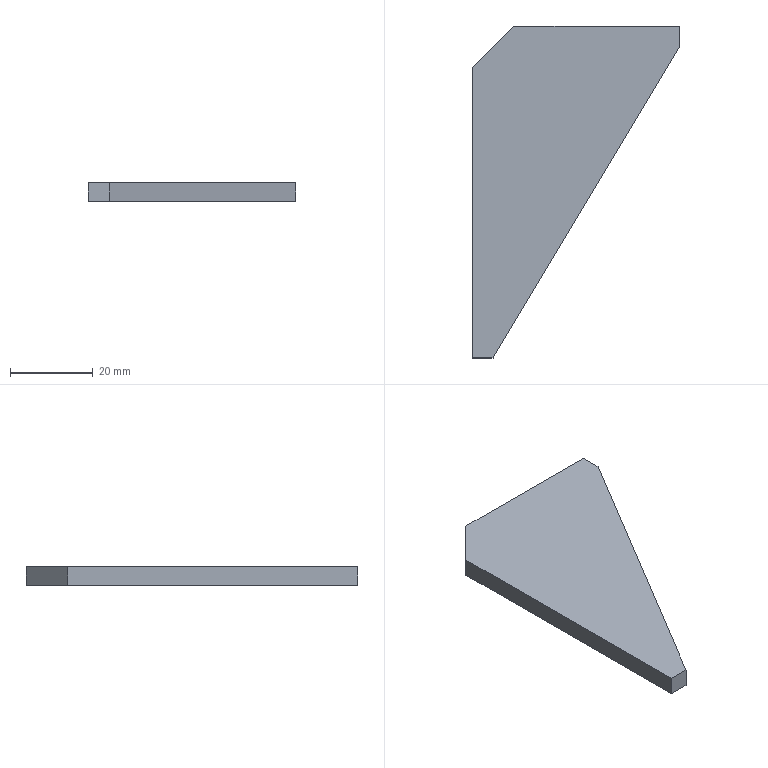Part | SolidWorks | features FlatPattern 1, SMBaseFlange 1, SheetMetal 1 | 1 solid | 8 faces | box 50 x 80 x 4.5 mm | volume 10181 mm3 | plane 8
STEP:
#1=CARTESIAN_POINT('',(0.,-5.,0.));
#2=VERTEX_POINT('',#1);
#3=CARTESIAN_POINT('',(0.,0.,0.));
#4=VERTEX_POINT('',#3);
#5=CARTESIAN_POINT('',(0.,-5.,0.));
#6=DIRECTION('',(0.,1.,0.));
#7=VECTOR('',#6,1000.);
#8=LINE('',#5,#7);
#9=EDGE_CURVE('',#2,#4,#8,.T.);
#10=ORIENTED_EDGE('',*,*,#9,.F.);
#11=CARTESIAN_POINT('',(0.,-5.,-4.5));
#12=VERTEX_POINT('',#11);
#13=CARTESIAN_POINT('',(0.,-5.,-4.5));
#14=DIRECTION('',(0.,0.,1.));
#15=VECTOR('',#14,1000.);
#16=LINE('',#13,#15);
#17=EDGE_CURVE('',#12,#2,#16,.T.);
#18=ORIENTED_EDGE('',*,*,#17,.F.);
#19=CARTESIAN_POINT('',(0.,0.,-4.5));
#20=VERTEX_POINT('',#19);
#21=CARTESIAN_POINT('',(0.,-5.,-4.5));
#22=DIRECTION('',(0.,1.,0.));
#23=VECTOR('',#22,1000.);
#24=LINE('',#21,#23);
#25=EDGE_CURVE('',#12,#20,#24,.T.);
#26=ORIENTED_EDGE('',*,*,#25,.T.);
#27=CARTESIAN_POINT('',(0.,0.,-4.5));
#28=DIRECTION('',(0.,0.,1.));
#29=VECTOR('',#28,1000.);
#30=LINE('',#27,#29);
#31=EDGE_CURVE('',#20,#4,#30,.T.);
#32=ORIENTED_EDGE('',*,*,#31,.T.);
#33=EDGE_LOOP('',(#10,#18,#26,#32));
#34=FACE_OUTER_BOUND('',#33,.T.);
#35=CARTESIAN_POINT('',(0.,-5.,-4.5));
#36=DIRECTION('',(1.,0.,0.));
#37=DIRECTION('',(0.,0.,-1.));
#38=AXIS2_PLACEMENT_3D('',#35,#36,#37);
#39=PLANE('',#38);
#40=ADVANCED_FACE('',(#34),#39,.T.);
#41=CARTESIAN_POINT('',(-45.,-80.,0.));
#42=VERTEX_POINT('',#41);
#43=CARTESIAN_POINT('',(-45.,-80.,0.));
#44=DIRECTION('',(0.5145,0.8575,0.));
#45=VECTOR('',#44,1000.);
#46=LINE('',#43,#45);
#47=EDGE_CURVE('',#42,#2,#46,.T.);
#48=ORIENTED_EDGE('',*,*,#47,.F.);
#49=CARTESIAN_POINT('',(-45.,-80.,-4.5));
#50=VERTEX_POINT('',#49);
#51=CARTESIAN_POINT('',(-45.,-80.,-4.5));
#52=DIRECTION('',(0.,0.,1.));
#53=VECTOR('',#52,1000.);
#54=LINE('',#51,#53);
#55=EDGE_CURVE('',#50,#42,#54,.T.);
#56=ORIENTED_EDGE('',*,*,#55,.F.);
#57=CARTESIAN_POINT('',(-45.,-80.,-4.5));
#58=DIRECTION('',(0.5145,0.8575,0.));
#59=VECTOR('',#58,1000.);
#60=LINE('',#57,#59);
#61=EDGE_CURVE('',#50,#12,#60,.T.);
#62=ORIENTED_EDGE('',*,*,#61,.T.);
#63=ORIENTED_EDGE('',*,*,#17,.T.);
#64=EDGE_LOOP('',(#48,#56,#62,#63));
#65=FACE_OUTER_BOUND('',#64,.T.);
#66=CARTESIAN_POINT('',(-45.,-80.,-4.5));
#67=DIRECTION('',(0.8575,-0.5145,0.));
#68=DIRECTION('',(0.5145,0.8575,0.));
#69=AXIS2_PLACEMENT_3D('',#66,#67,#68);
#70=PLANE('',#69);
#71=ADVANCED_FACE('',(#65),#70,.T.);
#72=CARTESIAN_POINT('',(-50.,-80.,0.));
#73=VERTEX_POINT('',#72);
#74=CARTESIAN_POINT('',(-50.,-80.,0.));
#75=DIRECTION('',(1.,0.,0.));
#76=VECTOR('',#75,1000.);
#77=LINE('',#74,#76);
#78=EDGE_CURVE('',#73,#42,#77,.T.);
#79=ORIENTED_EDGE('',*,*,#78,.F.);
#80=CARTESIAN_POINT('',(-50.,-80.,-4.5));
#81=VERTEX_POINT('',#80);
#82=CARTESIAN_POINT('',(-50.,-80.,-4.5));
#83=DIRECTION('',(0.,0.,1.));
#84=VECTOR('',#83,1000.);
#85=LINE('',#82,#84);
#86=EDGE_CURVE('',#81,#73,#85,.T.);
#87=ORIENTED_EDGE('',*,*,#86,.F.);
#88=CARTESIAN_POINT('',(-50.,-80.,-4.5));
#89=DIRECTION('',(1.,0.,0.));
#90=VECTOR('',#89,1000.);
#91=LINE('',#88,#90);
#92=EDGE_CURVE('',#81,#50,#91,.T.);
#93=ORIENTED_EDGE('',*,*,#92,.T.);
#94=ORIENTED_EDGE('',*,*,#55,.T.);
#95=EDGE_LOOP('',(#79,#87,#93,#94));
#96=FACE_OUTER_BOUND('',#95,.T.);
#97=CARTESIAN_POINT('',(-50.,-80.,-4.5));
#98=DIRECTION('',(0.,-1.,0.));
#99=DIRECTION('',(0.,0.,-1.));
#100=AXIS2_PLACEMENT_3D('',#97,#98,#99);
#101=PLANE('',#100);
#102=ADVANCED_FACE('',(#96),#101,.T.);
#103=CARTESIAN_POINT('',(-50.,-10.,0.));
#104=VERTEX_POINT('',#103);
#105=CARTESIAN_POINT('',(-50.,-10.,0.));
#106=DIRECTION('',(0.,-1.,0.));
#107=VECTOR('',#106,1000.);
#108=LINE('',#105,#107);
#109=EDGE_CURVE('',#104,#73,#108,.T.);
#110=ORIENTED_EDGE('',*,*,#109,.F.);
#111=CARTESIAN_POINT('',(-50.,-10.,-4.5));
#112=VERTEX_POINT('',#111);
#113=CARTESIAN_POINT('',(-50.,-10.,-4.5));
#114=DIRECTION('',(0.,0.,1.));
#115=VECTOR('',#114,1000.);
#116=LINE('',#113,#115);
#117=EDGE_CURVE('',#112,#104,#116,.T.);
#118=ORIENTED_EDGE('',*,*,#117,.F.);
#119=CARTESIAN_POINT('',(-50.,-10.,-4.5));
#120=DIRECTION('',(0.,-1.,0.));
#121=VECTOR('',#120,1000.);
#122=LINE('',#119,#121);
#123=EDGE_CURVE('',#112,#81,#122,.T.);
#124=ORIENTED_EDGE('',*,*,#123,.T.);
#125=ORIENTED_EDGE('',*,*,#86,.T.);
#126=EDGE_LOOP('',(#110,#118,#124,#125));
#127=FACE_OUTER_BOUND('',#126,.T.);
#128=CARTESIAN_POINT('',(-50.,-10.,-4.5));
#129=DIRECTION('',(-1.,0.,0.));
#130=DIRECTION('',(0.,-1.,0.));
#131=AXIS2_PLACEMENT_3D('',#128,#129,#130);
#132=PLANE('',#131);
#133=ADVANCED_FACE('',(#127),#132,.T.);
#134=CARTESIAN_POINT('',(-40.,0.,0.));
#135=VERTEX_POINT('',#134);
#136=CARTESIAN_POINT('',(-40.,0.,0.));
#137=DIRECTION('',(-0.7071,-0.7071,0.));
#138=VECTOR('',#137,1000.);
#139=LINE('',#136,#138);
#140=EDGE_CURVE('',#135,#104,#139,.T.);
#141=ORIENTED_EDGE('',*,*,#140,.F.);
#142=CARTESIAN_POINT('',(-40.,0.,-4.5));
#143=VERTEX_POINT('',#142);
#144=CARTESIAN_POINT('',(-40.,0.,-4.5));
#145=DIRECTION('',(0.,0.,1.));
#146=VECTOR('',#145,1000.);
#147=LINE('',#144,#146);
#148=EDGE_CURVE('',#143,#135,#147,.T.);
#149=ORIENTED_EDGE('',*,*,#148,.F.);
#150=CARTESIAN_POINT('',(-40.,0.,-4.5));
#151=DIRECTION('',(-0.7071,-0.7071,0.));
#152=VECTOR('',#151,1000.);
#153=LINE('',#150,#152);
#154=EDGE_CURVE('',#143,#112,#153,.T.);
#155=ORIENTED_EDGE('',*,*,#154,.T.);
#156=ORIENTED_EDGE('',*,*,#117,.T.);
#157=EDGE_LOOP('',(#141,#149,#155,#156));
#158=FACE_OUTER_BOUND('',#157,.T.);
#159=CARTESIAN_POINT('',(-40.,0.,-4.5));
#160=DIRECTION('',(-0.7071,0.7071,0.));
#161=DIRECTION('',(-0.7071,-0.7071,0.));
#162=AXIS2_PLACEMENT_3D('',#159,#160,#161);
#163=PLANE('',#162);
#164=ADVANCED_FACE('',(#158),#163,.T.);
#165=CARTESIAN_POINT('',(0.,0.,0.));
#166=DIRECTION('',(-1.,0.,0.));
#167=VECTOR('',#166,1000.);
#168=LINE('',#165,#167);
#169=EDGE_CURVE('',#4,#135,#168,.T.);
#170=ORIENTED_EDGE('',*,*,#169,.F.);
#171=ORIENTED_EDGE('',*,*,#31,.F.);
#172=CARTESIAN_POINT('',(0.,0.,-4.5));
#173=DIRECTION('',(-1.,0.,0.));
#174=VECTOR('',#173,1000.);
#175=LINE('',#172,#174);
#176=EDGE_CURVE('',#20,#143,#175,.T.);
#177=ORIENTED_EDGE('',*,*,#176,.T.);
#178=ORIENTED_EDGE('',*,*,#148,.T.);
#179=EDGE_LOOP('',(#170,#171,#177,#178));
#180=FACE_OUTER_BOUND('',#179,.T.);
#181=CARTESIAN_POINT('',(0.,0.,-4.5));
#182=DIRECTION('',(0.,1.,0.));
#183=DIRECTION('',(0.,0.,1.));
#184=AXIS2_PLACEMENT_3D('',#181,#182,#183);
#185=PLANE('',#184);
#186=ADVANCED_FACE('',(#180),#185,.T.);
#187=ORIENTED_EDGE('',*,*,#25,.F.);
#188=ORIENTED_EDGE('',*,*,#61,.F.);
#189=ORIENTED_EDGE('',*,*,#92,.F.);
#190=ORIENTED_EDGE('',*,*,#123,.F.);
#191=ORIENTED_EDGE('',*,*,#154,.F.);
#192=ORIENTED_EDGE('',*,*,#176,.F.);
#193=EDGE_LOOP('',(#187,#188,#189,#190,#191,#192));
#194=FACE_OUTER_BOUND('',#193,.T.);
#195=CARTESIAN_POINT('',(0.,0.,-4.5));
#196=DIRECTION('',(0.,0.,1.));
#197=DIRECTION('',(1.,0.,0.));
#198=AXIS2_PLACEMENT_3D('',#195,#196,#197);
#199=PLANE('',#198);
#200=ADVANCED_FACE('',(#194),#199,.F.);
#201=ORIENTED_EDGE('',*,*,#9,.T.);
#202=ORIENTED_EDGE('',*,*,#169,.T.);
#203=ORIENTED_EDGE('',*,*,#140,.T.);
#204=ORIENTED_EDGE('',*,*,#109,.T.);
#205=ORIENTED_EDGE('',*,*,#78,.T.);
#206=ORIENTED_EDGE('',*,*,#47,.T.);
#207=EDGE_LOOP('',(#201,#202,#203,#204,#205,#206));
#208=FACE_OUTER_BOUND('',#207,.T.);
#209=CARTESIAN_POINT('',(0.,0.,0.));
#210=DIRECTION('',(0.,0.,1.));
#211=DIRECTION('',(1.,0.,0.));
#212=AXIS2_PLACEMENT_3D('',#209,#210,#211);
#213=PLANE('',#212);
#214=ADVANCED_FACE('',(#208),#213,.T.);
#215=CLOSED_SHELL('',(#40,#71,#102,#133,#164,#186,#200,#214));
#216=MANIFOLD_SOLID_BREP('',#215);
#217=CARTESIAN_POINT('',(0.,0.,0.));
#218=DIRECTION('',(0.,0.,1.));
#219=DIRECTION('',(1.,0.,0.));
#220=AXIS2_PLACEMENT_3D('',#217,#218,#219);
#221=(LENGTH_UNIT()NAMED_UNIT(*)SI_UNIT(.MILLI.,.METRE.));
#222=UNCERTAINTY_MEASURE_WITH_UNIT(LENGTH_MEASURE(0.00001),#221,'','');
#223=(NAMED_UNIT(*)PLANE_ANGLE_UNIT()SI_UNIT($,.RADIAN.));
#224=(NAMED_UNIT(*)SI_UNIT($,.STERADIAN.)SOLID_ANGLE_UNIT());
#225=(GEOMETRIC_REPRESENTATION_CONTEXT(3)GLOBAL_UNCERTAINTY_ASSIGNED_CONTEXT((#222))GLOBAL_UNIT_ASSIGNED_CONTEXT((#221,#223,#224))REPRESENTATION_CONTEXT('',''));
#226=ADVANCED_BREP_SHAPE_REPRESENTATION('',(#216,#220),#225);